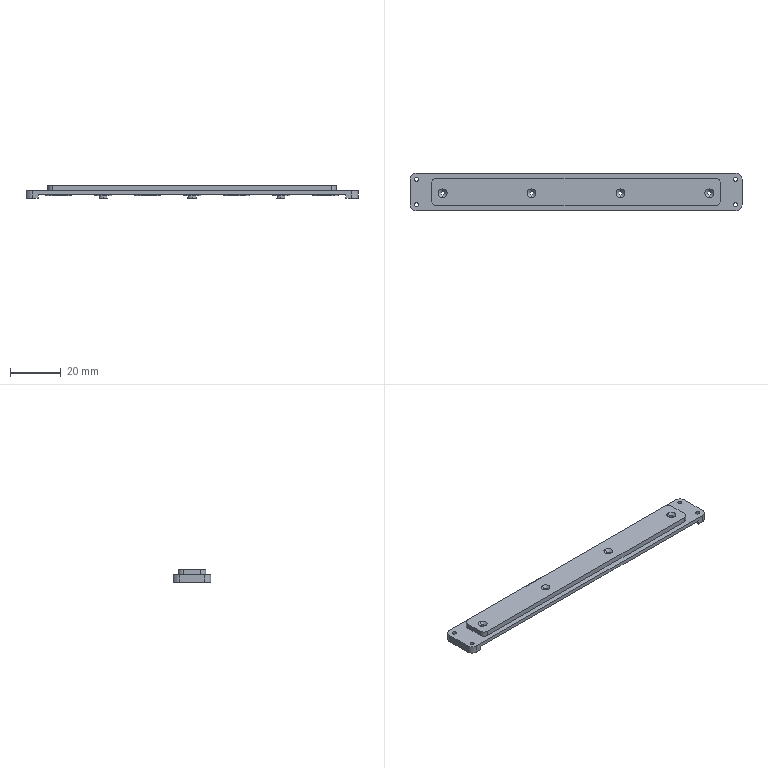NC program | NX | posted with a generic post | part box 130.666 x 14.95 x 5 mm
Lines 3663 to 3855 of 3855:
(PLANAR_MILL_COPY_COPY_COPY_COPY_COPY_COPY_1_COPY_1 , TOOL : D6A45)
N7288 T01 M6
N7290 G54
N7292 G17 G0 G90 X-58.394 Y1.27 S9500 M3
N7294 G43 Z30. H1
N7296 Z0.5
N7298 G94 G1 Z-1. F1250.
N7300 X-59.094 Y0.866
N7302 G3 X-59.594 Y0. R1.
N7304 G1 Y-7.375
N7306 G2 X-60.594 Y-8.375 R1.
N7308 G1 X-62.833
N7310 G2 X-66.233 Y-4.975 R3.4
N7312 G1 Y4.975
N7314 G2 X-62.833 Y8.375 R3.4
N7316 G1 X-60.594
N7318 G2 X-59.594 Y7.375 R1.
N7320 G1 Y0.
N7322 G3 X-59.094 Y-0.866 R1.
N7324 G1 X-58.394 Y-1.27
N7326 Z0.5
N7328 G0 Z30.
N7330 X58.406
N7332 Z0.5
N7334 G1 Z-1.
N7336 X59.106 Y-0.866
N7338 G3 X59.606 Y0. R1.
N7340 G1 Y7.375
N7342 G2 X60.606 Y8.375 R1.
N7344 G1 X62.833
N7346 G2 X66.233 Y4.975 R3.4
N7348 G1 Y-4.975
N7350 G2 X62.833 Y-8.375 R3.4
N7352 G1 X60.606
N7354 G2 X59.606 Y-7.375 R1.
N7356 G1 Y0.
N7358 G3 X59.106 Y0.866 R1.
N7360 G1 X58.406 Y1.27
N7362 Z0.5
N7364 G0 Z30.
(PLANAR_MILL_COPY_COPY_COPY_COPY_COPY_COPY_1_COPY_1_COPY , TOOL : D6A45)
N7366 X53.681 Y-1.27
N7368 Z-0.5
N7370 G1 Z-2.
N7372 X54.381 Y-0.866
N7374 G3 X54.881 Y0. R1.
N7376 G1 Y2.675
N7378 X54.893 Y2.74
N7380 X54.846 Y2.788
N7382 X54.781 Y2.775
N7384 X50.231
N7386 X50.166 Y2.788
N7388 X50.118 Y2.74
N7390 X50.131 Y2.675
N7392 Y-2.675
N7394 X50.118 Y-2.74
N7396 X50.166 Y-2.788
N7398 X50.231 Y-2.775
N7400 X54.781
N7402 X54.846 Y-2.788
N7404 X54.893 Y-2.74
N7406 X54.881 Y-2.675
N7408 Y0.
N7410 G3 X54.381 Y0.866 R1.
N7412 G1 X53.681 Y1.27
N7414 Z-0.5
N7416 G0 Z30.
N7418 X18.681 Y-1.27
N7420 Z-0.5
N7422 G1 Z-2.
N7424 X19.381 Y-0.866
N7426 G3 X19.881 Y0. R1.
N7428 G1 Y2.675
N7430 X19.893 Y2.74
N7432 X19.846 Y2.788
N7434 X19.781 Y2.775
N7436 X15.231
N7438 X15.166 Y2.788
N7440 X15.118 Y2.74
N7442 X15.131 Y2.675
N7444 Y-2.675
N7446 X15.118 Y-2.74
N7448 X15.166 Y-2.788
N7450 X15.231 Y-2.775
N7452 X19.781
N7454 X19.846 Y-2.788
N7456 X19.893 Y-2.74
N7458 X19.881 Y-2.675
N7460 Y0.
N7462 G3 X19.381 Y0.866 R1.
N7464 G1 X18.681 Y1.27
N7466 Z-0.5
N7468 G0 Z30.
N7470 X-16.319 Y-1.27
N7472 Z-0.5
N7474 G1 Z-2.
N7476 X-15.619 Y-0.866
N7478 G3 X-15.119 Y0. R1.
N7480 G1 Y2.675
N7482 X-15.107 Y2.74
N7484 X-15.154 Y2.788
N7486 X-15.219 Y2.775
N7488 X-19.769
N7490 X-19.834 Y2.788
N7492 X-19.882 Y2.74
N7494 X-19.869 Y2.675
N7496 Y-2.675
N7498 X-19.882 Y-2.74
N7500 X-19.834 Y-2.788
N7502 X-19.769 Y-2.775
N7504 X-15.219
N7506 X-15.154 Y-2.788
N7508 X-15.107 Y-2.74
N7510 X-15.119 Y-2.675
N7512 Y0.
N7514 G3 X-15.619 Y0.866 R1.
N7516 G1 X-16.319 Y1.27
N7518 Z-0.5
N7520 G0 Z30.
N7522 X-51.319 Y-1.27
N7524 Z-0.5
N7526 G1 Z-2.
N7528 X-50.619 Y-0.866
N7530 G3 X-50.119 Y0. R1.
N7532 G1 Y2.675
N7534 X-50.107 Y2.74
N7536 X-50.154 Y2.788
N7538 X-50.219 Y2.775
N7540 X-54.769
N7542 X-54.834 Y2.788
N7544 X-54.882 Y2.74
N7546 X-54.869 Y2.675
N7548 Y-2.675
N7550 X-54.882 Y-2.74
N7552 X-54.834 Y-2.788
N7554 X-54.769 Y-2.775
N7556 X-50.219
N7558 X-50.154 Y-2.788
N7560 X-50.107 Y-2.74
N7562 X-50.119 Y-2.675
N7564 Y0.
N7566 G3 X-50.619 Y0.866 R1.
N7568 G1 X-51.319 Y1.27
N7570 Z-0.5
N7572 G0 Z30.
(PLANAR_MILL_COPY_COPY_COPY_COPY_COPY_COPY_1_COPY_1_COPY_COPY , TOOL : D6A45)
N7574 X57.011 Y-9.804
N7576 Z-1.
N7578 G1 Z-2.5
N7580 X57.427 Y-9.351
N7582 G3 X57.644 Y-8.375 R1.
N7584 G1 X-57.632
N7586 G3 X-57.415 Y-9.351 R1.
N7588 G1 X-56.999 Y-9.804
N7590 Z-1.
N7592 G0 Z30.
N7594 Y9.804
N7596 Z-1.
N7598 G1 Z-2.5
N7600 X-57.415 Y9.351
N7602 G3 X-57.632 Y8.375 R1.
N7604 G1 X57.644
N7606 G3 X57.427 Y9.351 R1.
N7608 G1 X57.011 Y9.804
N7610 Z-1.
N7612 G0 Z30.
(DRILLING_COPY_1_COPY_1_COPY , TOOL : D6A45)
N7614 X62.833 Y-4.975 S5000
N7616 G81 G98 Z-1.1 F350. R3.
N7618 Y4.975
N7620 X-62.833
N7622 Y-4.975
N7624 G80
N7626 G0 X-62.833 Y-4.975 Z30.
(DRILLING_COPY_1_COPY_1_COPY_COPY , TOOL : D6A45)
N7628 X-34.994 Y0.
N7630 G81 Z-1.1 F350. R3.
N7632 X0.006
N7634 X35.006
N7636 G80
N7638 G0 X35.006 Y0. Z30.
N7640 M5
N7642 M2